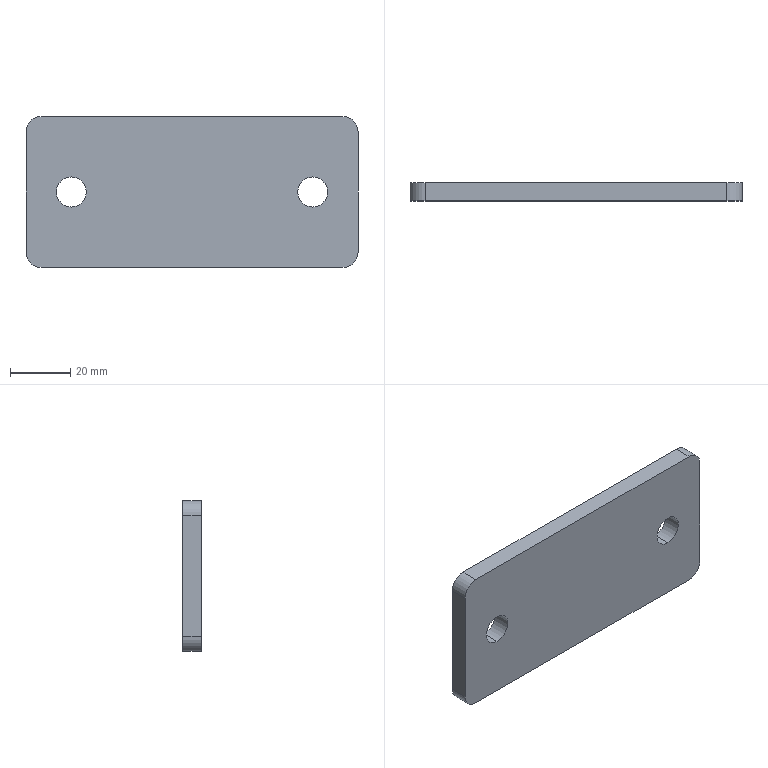Part | SolidWorks | features EdgeFlange 2, Fillet 2, HoleWzd 2, FlatPattern 1, SMBaseFlange 1, SheetMetal 1 | 1 solid | 14 faces | box 110 x 6 x 50 mm | volume 31929 mm3 | cylinder 8 | plane 6 | commonest cylinder face diameters 10 x8
STEP:
#1=CARTESIAN_POINT('',(-40.,0.,5.));
#2=VERTEX_POINT('',#1);
#3=CARTESIAN_POINT('',(-40.,0.,-5.));
#4=VERTEX_POINT('',#3);
#5=CARTESIAN_POINT('',(-40.,0.,0.));
#6=DIRECTION('',(0.,-1.,0.));
#7=DIRECTION('',(0.,0.,-1.));
#8=AXIS2_PLACEMENT_3D('',#5,#6,#7);
#9=CIRCLE('',#8,5.);
#10=EDGE_CURVE('',#2,#4,#9,.T.);
#11=ORIENTED_EDGE('',*,*,#10,.F.);
#12=CARTESIAN_POINT('',(-40.,-6.,5.));
#13=VERTEX_POINT('',#12);
#14=CARTESIAN_POINT('',(-40.,-6.,5.));
#15=DIRECTION('',(0.,-1.,0.));
#16=VECTOR('',#15,1000.);
#17=LINE('',#14,#16);
#18=EDGE_CURVE('',#2,#13,#17,.T.);
#19=ORIENTED_EDGE('',*,*,#18,.T.);
#20=CARTESIAN_POINT('',(-40.,-6.,-5.));
#21=VERTEX_POINT('',#20);
#22=CARTESIAN_POINT('',(-40.,-6.,0.));
#23=DIRECTION('',(0.,-1.,0.));
#24=DIRECTION('',(0.,0.,-1.));
#25=AXIS2_PLACEMENT_3D('',#22,#23,#24);
#26=CIRCLE('',#25,5.);
#27=EDGE_CURVE('',#13,#21,#26,.T.);
#28=ORIENTED_EDGE('',*,*,#27,.T.);
#29=CARTESIAN_POINT('',(-40.,-6.,-5.));
#30=DIRECTION('',(0.,-1.,0.));
#31=VECTOR('',#30,1000.);
#32=LINE('',#29,#31);
#33=EDGE_CURVE('',#4,#21,#32,.T.);
#34=ORIENTED_EDGE('',*,*,#33,.F.);
#35=EDGE_LOOP('',(#11,#19,#28,#34));
#36=FACE_OUTER_BOUND('',#35,.T.);
#37=CARTESIAN_POINT('',(-40.,-6.,0.));
#38=DIRECTION('',(0.,-1.,0.));
#39=DIRECTION('',(0.,0.,-1.));
#40=AXIS2_PLACEMENT_3D('',#37,#38,#39);
#41=CYLINDRICAL_SURFACE('',#40,5.);
#42=ADVANCED_FACE('',(#36),#41,.F.);
#43=CARTESIAN_POINT('',(40.,0.,5.));
#44=VERTEX_POINT('',#43);
#45=CARTESIAN_POINT('',(40.,0.,-5.));
#46=VERTEX_POINT('',#45);
#47=CARTESIAN_POINT('',(40.,0.,0.));
#48=DIRECTION('',(0.,-1.,0.));
#49=DIRECTION('',(0.,0.,-1.));
#50=AXIS2_PLACEMENT_3D('',#47,#48,#49);
#51=CIRCLE('',#50,5.);
#52=EDGE_CURVE('',#44,#46,#51,.T.);
#53=ORIENTED_EDGE('',*,*,#52,.F.);
#54=CARTESIAN_POINT('',(40.,-6.,5.));
#55=VERTEX_POINT('',#54);
#56=CARTESIAN_POINT('',(40.,-6.,5.));
#57=DIRECTION('',(0.,-1.,0.));
#58=VECTOR('',#57,1000.);
#59=LINE('',#56,#58);
#60=EDGE_CURVE('',#44,#55,#59,.T.);
#61=ORIENTED_EDGE('',*,*,#60,.T.);
#62=CARTESIAN_POINT('',(40.,-6.,-5.));
#63=VERTEX_POINT('',#62);
#64=CARTESIAN_POINT('',(40.,-6.,0.));
#65=DIRECTION('',(0.,-1.,0.));
#66=DIRECTION('',(0.,0.,-1.));
#67=AXIS2_PLACEMENT_3D('',#64,#65,#66);
#68=CIRCLE('',#67,5.);
#69=EDGE_CURVE('',#55,#63,#68,.T.);
#70=ORIENTED_EDGE('',*,*,#69,.T.);
#71=CARTESIAN_POINT('',(40.,-6.,-5.));
#72=DIRECTION('',(0.,-1.,0.));
#73=VECTOR('',#72,1000.);
#74=LINE('',#71,#73);
#75=EDGE_CURVE('',#46,#63,#74,.T.);
#76=ORIENTED_EDGE('',*,*,#75,.F.);
#77=EDGE_LOOP('',(#53,#61,#70,#76));
#78=FACE_OUTER_BOUND('',#77,.T.);
#79=CARTESIAN_POINT('',(40.,-6.,0.));
#80=DIRECTION('',(0.,-1.,0.));
#81=DIRECTION('',(0.,0.,-1.));
#82=AXIS2_PLACEMENT_3D('',#79,#80,#81);
#83=CYLINDRICAL_SURFACE('',#82,5.);
#84=ADVANCED_FACE('',(#78),#83,.F.);
#85=CARTESIAN_POINT('',(55.,-6.,20.));
#86=VERTEX_POINT('',#85);
#87=CARTESIAN_POINT('',(55.,-6.,-20.));
#88=VERTEX_POINT('',#87);
#89=CARTESIAN_POINT('',(55.,-6.,-25.));
#90=DIRECTION('',(0.,0.,-1.));
#91=VECTOR('',#90,1000.);
#92=LINE('',#89,#91);
#93=EDGE_CURVE('',#86,#88,#92,.T.);
#94=ORIENTED_EDGE('',*,*,#93,.T.);
#95=CARTESIAN_POINT('',(55.,0.,-20.));
#96=VERTEX_POINT('',#95);
#97=CARTESIAN_POINT('',(55.,-6.,-20.));
#98=DIRECTION('',(0.,1.,0.));
#99=VECTOR('',#98,1000.);
#100=LINE('',#97,#99);
#101=EDGE_CURVE('',#88,#96,#100,.T.);
#102=ORIENTED_EDGE('',*,*,#101,.T.);
#103=CARTESIAN_POINT('',(55.,0.,20.));
#104=VERTEX_POINT('',#103);
#105=CARTESIAN_POINT('',(55.,0.,-25.));
#106=DIRECTION('',(0.,0.,-1.));
#107=VECTOR('',#106,1000.);
#108=LINE('',#105,#107);
#109=EDGE_CURVE('',#104,#96,#108,.T.);
#110=ORIENTED_EDGE('',*,*,#109,.F.);
#111=CARTESIAN_POINT('',(55.,-6.,20.));
#112=DIRECTION('',(0.,-1.,0.));
#113=VECTOR('',#112,1000.);
#114=LINE('',#111,#113);
#115=EDGE_CURVE('',#104,#86,#114,.T.);
#116=ORIENTED_EDGE('',*,*,#115,.T.);
#117=EDGE_LOOP('',(#94,#102,#110,#116));
#118=FACE_OUTER_BOUND('',#117,.T.);
#119=CARTESIAN_POINT('',(55.,-6.,-25.));
#120=DIRECTION('',(1.,0.,0.));
#121=DIRECTION('',(0.,0.,-1.));
#122=AXIS2_PLACEMENT_3D('',#119,#120,#121);
#123=PLANE('',#122);
#124=ADVANCED_FACE('',(#118),#123,.T.);
#125=CARTESIAN_POINT('',(-50.,-6.,25.));
#126=VERTEX_POINT('',#125);
#127=CARTESIAN_POINT('',(50.,-6.,25.));
#128=VERTEX_POINT('',#127);
#129=CARTESIAN_POINT('',(-55.,-6.,25.));
#130=DIRECTION('',(1.,0.,0.));
#131=VECTOR('',#130,1000.);
#132=LINE('',#129,#131);
#133=EDGE_CURVE('',#126,#128,#132,.T.);
#134=ORIENTED_EDGE('',*,*,#133,.T.);
#135=CARTESIAN_POINT('',(50.,0.,25.));
#136=VERTEX_POINT('',#135);
#137=CARTESIAN_POINT('',(50.,-6.,25.));
#138=DIRECTION('',(0.,1.,0.));
#139=VECTOR('',#138,1000.);
#140=LINE('',#137,#139);
#141=EDGE_CURVE('',#128,#136,#140,.T.);
#142=ORIENTED_EDGE('',*,*,#141,.T.);
#143=CARTESIAN_POINT('',(-50.,0.,25.));
#144=VERTEX_POINT('',#143);
#145=CARTESIAN_POINT('',(-55.,0.,25.));
#146=DIRECTION('',(1.,0.,0.));
#147=VECTOR('',#146,1000.);
#148=LINE('',#145,#147);
#149=EDGE_CURVE('',#144,#136,#148,.T.);
#150=ORIENTED_EDGE('',*,*,#149,.F.);
#151=CARTESIAN_POINT('',(-50.,-6.,25.));
#152=DIRECTION('',(0.,-1.,0.));
#153=VECTOR('',#152,1000.);
#154=LINE('',#151,#153);
#155=EDGE_CURVE('',#144,#126,#154,.T.);
#156=ORIENTED_EDGE('',*,*,#155,.T.);
#157=EDGE_LOOP('',(#134,#142,#150,#156));
#158=FACE_OUTER_BOUND('',#157,.T.);
#159=CARTESIAN_POINT('',(-55.,-6.,25.));
#160=DIRECTION('',(0.,0.,1.));
#161=DIRECTION('',(1.,0.,0.));
#162=AXIS2_PLACEMENT_3D('',#159,#160,#161);
#163=PLANE('',#162);
#164=ADVANCED_FACE('',(#158),#163,.T.);
#165=CARTESIAN_POINT('',(-55.,0.,-20.));
#166=VERTEX_POINT('',#165);
#167=CARTESIAN_POINT('',(-55.,0.,20.));
#168=VERTEX_POINT('',#167);
#169=CARTESIAN_POINT('',(-55.,0.,-25.));
#170=DIRECTION('',(0.,0.,1.));
#171=VECTOR('',#170,1000.);
#172=LINE('',#169,#171);
#173=EDGE_CURVE('',#166,#168,#172,.T.);
#174=ORIENTED_EDGE('',*,*,#173,.F.);
#175=CARTESIAN_POINT('',(-55.,-6.,-20.));
#176=VERTEX_POINT('',#175);
#177=CARTESIAN_POINT('',(-55.,-6.,-20.));
#178=DIRECTION('',(0.,-1.,0.));
#179=VECTOR('',#178,1000.);
#180=LINE('',#177,#179);
#181=EDGE_CURVE('',#166,#176,#180,.T.);
#182=ORIENTED_EDGE('',*,*,#181,.T.);
#183=CARTESIAN_POINT('',(-55.,-6.,20.));
#184=VERTEX_POINT('',#183);
#185=CARTESIAN_POINT('',(-55.,-6.,-25.));
#186=DIRECTION('',(0.,0.,1.));
#187=VECTOR('',#186,1000.);
#188=LINE('',#185,#187);
#189=EDGE_CURVE('',#176,#184,#188,.T.);
#190=ORIENTED_EDGE('',*,*,#189,.T.);
#191=CARTESIAN_POINT('',(-55.,-6.,20.));
#192=DIRECTION('',(0.,1.,0.));
#193=VECTOR('',#192,1000.);
#194=LINE('',#191,#193);
#195=EDGE_CURVE('',#184,#168,#194,.T.);
#196=ORIENTED_EDGE('',*,*,#195,.T.);
#197=EDGE_LOOP('',(#174,#182,#190,#196));
#198=FACE_OUTER_BOUND('',#197,.T.);
#199=CARTESIAN_POINT('',(-55.,-6.,-25.));
#200=DIRECTION('',(-1.,0.,0.));
#201=DIRECTION('',(0.,0.,1.));
#202=AXIS2_PLACEMENT_3D('',#199,#200,#201);
#203=PLANE('',#202);
#204=ADVANCED_FACE('',(#198),#203,.T.);
#205=CARTESIAN_POINT('',(50.,0.,-25.));
#206=VERTEX_POINT('',#205);
#207=CARTESIAN_POINT('',(-50.,0.,-25.));
#208=VERTEX_POINT('',#207);
#209=CARTESIAN_POINT('',(-55.,0.,-25.));
#210=DIRECTION('',(-1.,0.,0.));
#211=VECTOR('',#210,1000.);
#212=LINE('',#209,#211);
#213=EDGE_CURVE('',#206,#208,#212,.T.);
#214=ORIENTED_EDGE('',*,*,#213,.F.);
#215=CARTESIAN_POINT('',(50.,-6.,-25.));
#216=VERTEX_POINT('',#215);
#217=CARTESIAN_POINT('',(50.,-6.,-25.));
#218=DIRECTION('',(0.,-1.,0.));
#219=VECTOR('',#218,1000.);
#220=LINE('',#217,#219);
#221=EDGE_CURVE('',#206,#216,#220,.T.);
#222=ORIENTED_EDGE('',*,*,#221,.T.);
#223=CARTESIAN_POINT('',(-50.,-6.,-25.));
#224=VERTEX_POINT('',#223);
#225=CARTESIAN_POINT('',(-55.,-6.,-25.));
#226=DIRECTION('',(-1.,0.,0.));
#227=VECTOR('',#226,1000.);
#228=LINE('',#225,#227);
#229=EDGE_CURVE('',#216,#224,#228,.T.);
#230=ORIENTED_EDGE('',*,*,#229,.T.);
#231=CARTESIAN_POINT('',(-50.,-6.,-25.));
#232=DIRECTION('',(0.,1.,0.));
#233=VECTOR('',#232,1000.);
#234=LINE('',#231,#233);
#235=EDGE_CURVE('',#224,#208,#234,.T.);
#236=ORIENTED_EDGE('',*,*,#235,.T.);
#237=EDGE_LOOP('',(#214,#222,#230,#236));
#238=FACE_OUTER_BOUND('',#237,.T.);
#239=CARTESIAN_POINT('',(-55.,-6.,-25.));
#240=DIRECTION('',(0.,0.,-1.));
#241=DIRECTION('',(-1.,0.,0.));
#242=AXIS2_PLACEMENT_3D('',#239,#240,#241);
#243=PLANE('',#242);
#244=ADVANCED_FACE('',(#238),#243,.T.);
#245=CARTESIAN_POINT('',(-40.,-6.,0.));
#246=DIRECTION('',(0.,-1.,0.));
#247=DIRECTION('',(0.,0.,-1.));
#248=AXIS2_PLACEMENT_3D('',#245,#246,#247);
#249=CIRCLE('',#248,5.);
#250=EDGE_CURVE('',#21,#13,#249,.T.);
#251=ORIENTED_EDGE('',*,*,#250,.F.);
#252=ORIENTED_EDGE('',*,*,#27,.F.);
#253=EDGE_LOOP('',(#251,#252));
#254=FACE_BOUND('',#253,.T.);
#255=CARTESIAN_POINT('',(40.,-6.,0.));
#256=DIRECTION('',(0.,-1.,0.));
#257=DIRECTION('',(0.,0.,-1.));
#258=AXIS2_PLACEMENT_3D('',#255,#256,#257);
#259=CIRCLE('',#258,5.);
#260=EDGE_CURVE('',#63,#55,#259,.T.);
#261=ORIENTED_EDGE('',*,*,#260,.F.);
#262=ORIENTED_EDGE('',*,*,#69,.F.);
#263=EDGE_LOOP('',(#261,#262));
#264=FACE_BOUND('',#263,.T.);
#265=ORIENTED_EDGE('',*,*,#229,.F.);
#266=CARTESIAN_POINT('',(50.,-6.,-20.));
#267=DIRECTION('',(0.,-1.,0.));
#268=DIRECTION('',(0.,0.,1.));
#269=AXIS2_PLACEMENT_3D('',#266,#267,#268);
#270=CIRCLE('',#269,5.);
#271=EDGE_CURVE('',#216,#88,#270,.T.);
#272=ORIENTED_EDGE('',*,*,#271,.T.);
#273=ORIENTED_EDGE('',*,*,#93,.F.);
#274=CARTESIAN_POINT('',(50.,-6.,20.));
#275=DIRECTION('',(0.,-1.,0.));
#276=DIRECTION('',(0.,0.,1.));
#277=AXIS2_PLACEMENT_3D('',#274,#275,#276);
#278=CIRCLE('',#277,5.);
#279=EDGE_CURVE('',#86,#128,#278,.T.);
#280=ORIENTED_EDGE('',*,*,#279,.T.);
#281=ORIENTED_EDGE('',*,*,#133,.F.);
#282=CARTESIAN_POINT('',(-50.,-6.,20.));
#283=DIRECTION('',(0.,-1.,0.));
#284=DIRECTION('',(0.,0.,1.));
#285=AXIS2_PLACEMENT_3D('',#282,#283,#284);
#286=CIRCLE('',#285,5.);
#287=EDGE_CURVE('',#126,#184,#286,.T.);
#288=ORIENTED_EDGE('',*,*,#287,.T.);
#289=ORIENTED_EDGE('',*,*,#189,.F.);
#290=CARTESIAN_POINT('',(-50.,-6.,-20.));
#291=DIRECTION('',(0.,-1.,0.));
#292=DIRECTION('',(0.,0.,1.));
#293=AXIS2_PLACEMENT_3D('',#290,#291,#292);
#294=CIRCLE('',#293,5.);
#295=EDGE_CURVE('',#176,#224,#294,.T.);
#296=ORIENTED_EDGE('',*,*,#295,.T.);
#297=EDGE_LOOP('',(#265,#272,#273,#280,#281,#288,#289,#296));
#298=FACE_OUTER_BOUND('',#297,.T.);
#299=CARTESIAN_POINT('',(0.,-6.,0.));
#300=DIRECTION('',(0.,1.,0.));
#301=DIRECTION('',(0.,0.,1.));
#302=AXIS2_PLACEMENT_3D('',#299,#300,#301);
#303=PLANE('',#302);
#304=ADVANCED_FACE('',(#254,#264,#298),#303,.F.);
#305=CARTESIAN_POINT('',(-40.,0.,0.));
#306=DIRECTION('',(0.,-1.,0.));
#307=DIRECTION('',(0.,0.,-1.));
#308=AXIS2_PLACEMENT_3D('',#305,#306,#307);
#309=CIRCLE('',#308,5.);
#310=EDGE_CURVE('',#4,#2,#309,.T.);
#311=ORIENTED_EDGE('',*,*,#310,.T.);
#312=ORIENTED_EDGE('',*,*,#10,.T.);
#313=EDGE_LOOP('',(#311,#312));
#314=FACE_BOUND('',#313,.T.);
#315=CARTESIAN_POINT('',(40.,0.,0.));
#316=DIRECTION('',(0.,-1.,0.));
#317=DIRECTION('',(0.,0.,-1.));
#318=AXIS2_PLACEMENT_3D('',#315,#316,#317);
#319=CIRCLE('',#318,5.);
#320=EDGE_CURVE('',#46,#44,#319,.T.);
#321=ORIENTED_EDGE('',*,*,#320,.T.);
#322=ORIENTED_EDGE('',*,*,#52,.T.);
#323=EDGE_LOOP('',(#321,#322));
#324=FACE_BOUND('',#323,.T.);
#325=ORIENTED_EDGE('',*,*,#109,.T.);
#326=CARTESIAN_POINT('',(50.,0.,-20.));
#327=DIRECTION('',(0.,1.,0.));
#328=DIRECTION('',(0.,0.,1.));
#329=AXIS2_PLACEMENT_3D('',#326,#327,#328);
#330=CIRCLE('',#329,5.);
#331=EDGE_CURVE('',#96,#206,#330,.T.);
#332=ORIENTED_EDGE('',*,*,#331,.T.);
#333=ORIENTED_EDGE('',*,*,#213,.T.);
#334=CARTESIAN_POINT('',(-50.,0.,-20.));
#335=DIRECTION('',(0.,1.,0.));
#336=DIRECTION('',(0.,0.,1.));
#337=AXIS2_PLACEMENT_3D('',#334,#335,#336);
#338=CIRCLE('',#337,5.);
#339=EDGE_CURVE('',#208,#166,#338,.T.);
#340=ORIENTED_EDGE('',*,*,#339,.T.);
#341=ORIENTED_EDGE('',*,*,#173,.T.);
#342=CARTESIAN_POINT('',(-50.,0.,20.));
#343=DIRECTION('',(0.,1.,0.));
#344=DIRECTION('',(0.,0.,1.));
#345=AXIS2_PLACEMENT_3D('',#342,#343,#344);
#346=CIRCLE('',#345,5.);
#347=EDGE_CURVE('',#168,#144,#346,.T.);
#348=ORIENTED_EDGE('',*,*,#347,.T.);
#349=ORIENTED_EDGE('',*,*,#149,.T.);
#350=CARTESIAN_POINT('',(50.,0.,20.));
#351=DIRECTION('',(0.,1.,0.));
#352=DIRECTION('',(0.,0.,1.));
#353=AXIS2_PLACEMENT_3D('',#350,#351,#352);
#354=CIRCLE('',#353,5.);
#355=EDGE_CURVE('',#136,#104,#354,.T.);
#356=ORIENTED_EDGE('',*,*,#355,.T.);
#357=EDGE_LOOP('',(#325,#332,#333,#340,#341,#348,#349,#356));
#358=FACE_OUTER_BOUND('',#357,.T.);
#359=CARTESIAN_POINT('',(0.,0.,0.));
#360=DIRECTION('',(0.,1.,0.));
#361=DIRECTION('',(0.,0.,1.));
#362=AXIS2_PLACEMENT_3D('',#359,#360,#361);
#363=PLANE('',#362);
#364=ADVANCED_FACE('',(#314,#324,#358),#363,.T.);
#365=ORIENTED_EDGE('',*,*,#60,.F.);
#366=ORIENTED_EDGE('',*,*,#320,.F.);
#367=ORIENTED_EDGE('',*,*,#75,.T.);
#368=ORIENTED_EDGE('',*,*,#260,.T.);
#369=EDGE_LOOP('',(#365,#366,#367,#368));
#370=FACE_OUTER_BOUND('',#369,.T.);
#371=CARTESIAN_POINT('',(40.,-6.,0.));
#372=DIRECTION('',(0.,-1.,0.));
#373=DIRECTION('',(0.,0.,-1.));
#374=AXIS2_PLACEMENT_3D('',#371,#372,#373);
#375=CYLINDRICAL_SURFACE('',#374,5.);
#376=ADVANCED_FACE('',(#370),#375,.F.);
#377=ORIENTED_EDGE('',*,*,#18,.F.);
#378=ORIENTED_EDGE('',*,*,#310,.F.);
#379=ORIENTED_EDGE('',*,*,#33,.T.);
#380=ORIENTED_EDGE('',*,*,#250,.T.);
#381=EDGE_LOOP('',(#377,#378,#379,#380));
#382=FACE_OUTER_BOUND('',#381,.T.);
#383=CARTESIAN_POINT('',(-40.,-6.,0.));
#384=DIRECTION('',(0.,-1.,0.));
#385=DIRECTION('',(0.,0.,-1.));
#386=AXIS2_PLACEMENT_3D('',#383,#384,#385);
#387=CYLINDRICAL_SURFACE('',#386,5.);
#388=ADVANCED_FACE('',(#382),#387,.F.);
#389=ORIENTED_EDGE('',*,*,#271,.F.);
#390=ORIENTED_EDGE('',*,*,#221,.F.);
#391=ORIENTED_EDGE('',*,*,#331,.F.);
#392=ORIENTED_EDGE('',*,*,#101,.F.);
#393=EDGE_LOOP('',(#389,#390,#391,#392));
#394=FACE_OUTER_BOUND('',#393,.T.);
#395=CARTESIAN_POINT('',(50.,-6.,-20.));
#396=DIRECTION('',(0.,1.,0.));
#397=DIRECTION('',(0.,0.,1.));
#398=AXIS2_PLACEMENT_3D('',#395,#396,#397);
#399=CYLINDRICAL_SURFACE('',#398,5.);
#400=ADVANCED_FACE('',(#394),#399,.T.);
#401=ORIENTED_EDGE('',*,*,#279,.F.);
#402=ORIENTED_EDGE('',*,*,#115,.F.);
#403=ORIENTED_EDGE('',*,*,#355,.F.);
#404=ORIENTED_EDGE('',*,*,#141,.F.);
#405=EDGE_LOOP('',(#401,#402,#403,#404));
#406=FACE_OUTER_BOUND('',#405,.T.);
#407=CARTESIAN_POINT('',(50.,-6.,20.));
#408=DIRECTION('',(0.,1.,0.));
#409=DIRECTION('',(0.,0.,1.));
#410=AXIS2_PLACEMENT_3D('',#407,#408,#409);
#411=CYLINDRICAL_SURFACE('',#410,5.);
#412=ADVANCED_FACE('',(#406),#411,.T.);
#413=ORIENTED_EDGE('',*,*,#295,.F.);
#414=ORIENTED_EDGE('',*,*,#181,.F.);
#415=ORIENTED_EDGE('',*,*,#339,.F.);
#416=ORIENTED_EDGE('',*,*,#235,.F.);
#417=EDGE_LOOP('',(#413,#414,#415,#416));
#418=FACE_OUTER_BOUND('',#417,.T.);
#419=CARTESIAN_POINT('',(-50.,-6.,-20.));
#420=DIRECTION('',(0.,1.,0.));
#421=DIRECTION('',(0.,0.,1.));
#422=AXIS2_PLACEMENT_3D('',#419,#420,#421);
#423=CYLINDRICAL_SURFACE('',#422,5.);
#424=ADVANCED_FACE('',(#418),#423,.T.);
#425=ORIENTED_EDGE('',*,*,#287,.F.);
#426=ORIENTED_EDGE('',*,*,#155,.F.);
#427=ORIENTED_EDGE('',*,*,#347,.F.);
#428=ORIENTED_EDGE('',*,*,#195,.F.);
#429=EDGE_LOOP('',(#425,#426,#427,#428));
#430=FACE_OUTER_BOUND('',#429,.T.);
#431=CARTESIAN_POINT('',(-50.,-6.,20.));
#432=DIRECTION('',(0.,1.,0.));
#433=DIRECTION('',(0.,0.,1.));
#434=AXIS2_PLACEMENT_3D('',#431,#432,#433);
#435=CYLINDRICAL_SURFACE('',#434,5.);
#436=ADVANCED_FACE('',(#430),#435,.T.);
#437=CLOSED_SHELL('',(#42,#84,#124,#164,#204,#244,#304,#364,#376,#388,#400,#412,#424,#436));
#438=MANIFOLD_SOLID_BREP('',#437);
#439=CARTESIAN_POINT('',(0.,0.,0.));
#440=DIRECTION('',(0.,0.,1.));
#441=DIRECTION('',(1.,0.,0.));
#442=AXIS2_PLACEMENT_3D('',#439,#440,#441);
#443=(LENGTH_UNIT()NAMED_UNIT(*)SI_UNIT(.MILLI.,.METRE.));
#444=UNCERTAINTY_MEASURE_WITH_UNIT(LENGTH_MEASURE(0.00001),#443,'','');
#445=(NAMED_UNIT(*)PLANE_ANGLE_UNIT()SI_UNIT($,.RADIAN.));
#446=(NAMED_UNIT(*)SI_UNIT($,.STERADIAN.)SOLID_ANGLE_UNIT());
#447=(GEOMETRIC_REPRESENTATION_CONTEXT(3)GLOBAL_UNCERTAINTY_ASSIGNED_CONTEXT((#444))GLOBAL_UNIT_ASSIGNED_CONTEXT((#443,#445,#446))REPRESENTATION_CONTEXT('',''));
#448=ADVANCED_BREP_SHAPE_REPRESENTATION('',(#438,#442),#447);